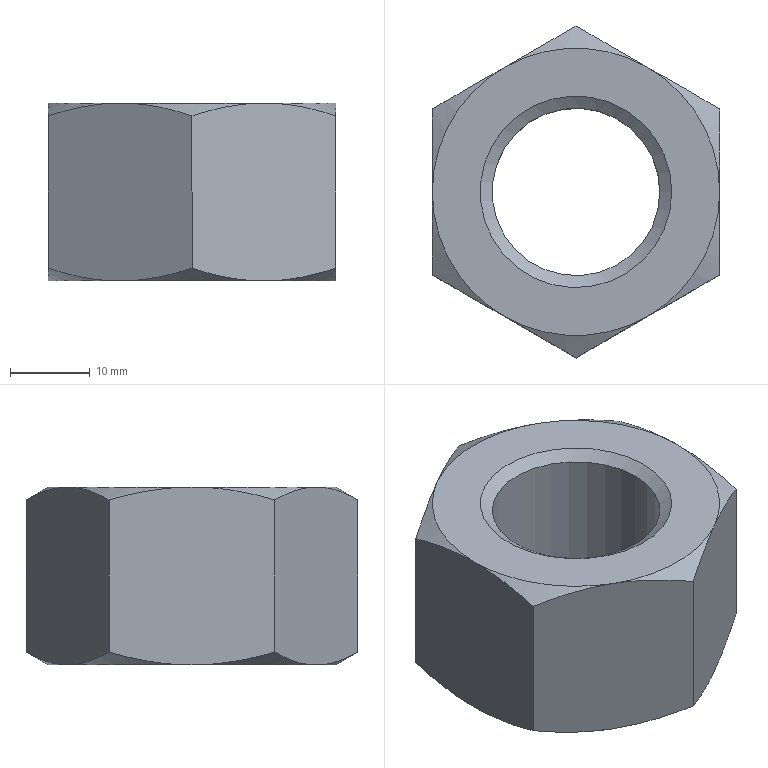Part | NX | features Hexagon Nut ISO - 4034 - M24 - N_Hexagon Nut ISO - 4034 - M24 - N 2 | 1 solid | 24 faces | box 36 x 41.569 x 22.3 mm | volume 17091 mm3 | cone 14 | plane 8 | cylinder 2 | commonest cylinder face diameters 21 x1 24 x1
STEP:
#1=CARTESIAN_POINT('',(9.,15.588,-22.3));
#2=VERTEX_POINT('',#1);
#3=CARTESIAN_POINT('',(18.,10.392,-20.692));
#4=VERTEX_POINT('',#3);
#5=CARTESIAN_POINT('',(9.,15.588,-22.3));
#6=CARTESIAN_POINT('',(12.072,13.815,-22.3));
#7=CARTESIAN_POINT('',(15.06,12.09,-21.672));
#8=CARTESIAN_POINT('',(18.,10.392,-20.692));
#9=B_SPLINE_CURVE_WITH_KNOTS('',3,(#5,#6,#7,#8),.UNSPECIFIED.,.F.,.F.,(4,4),(0.,0.01052),.UNSPECIFIED.);
#10=EDGE_CURVE('',#2,#4,#9,.T.);
#11=ORIENTED_EDGE('',*,*,#10,.F.);
#12=CARTESIAN_POINT('',(-0.000000038,20.785,-20.692));
#13=VERTEX_POINT('',#12);
#14=CARTESIAN_POINT('',(-0.000000042,20.785,-20.692));
#15=CARTESIAN_POINT('',(2.94,19.087,-21.672));
#16=CARTESIAN_POINT('',(5.928,17.362,-22.3));
#17=CARTESIAN_POINT('',(9.,15.588,-22.3));
#18=B_SPLINE_CURVE_WITH_KNOTS('',3,(#14,#15,#16,#17),.UNSPECIFIED.,.F.,.F.,(4,4),(0.,0.01052),.UNSPECIFIED.);
#19=EDGE_CURVE('',#13,#2,#18,.T.);
#20=ORIENTED_EDGE('',*,*,#19,.F.);
#21=CARTESIAN_POINT('',(0.000000012,20.785,-1.608));
#22=VERTEX_POINT('',#21);
#23=CARTESIAN_POINT('',(0.,20.785,-22.3));
#24=DIRECTION('',(0.,0.,1.));
#25=VECTOR('',#24,1000.);
#26=LINE('',#23,#25);
#27=EDGE_CURVE('',#22,#13,#26,.F.);
#28=ORIENTED_EDGE('',*,*,#27,.F.);
#29=CARTESIAN_POINT('',(9.,15.588,0.));
#30=VERTEX_POINT('',#29);
#31=CARTESIAN_POINT('',(9.,15.588,0.));
#32=CARTESIAN_POINT('',(5.928,17.362,0.));
#33=CARTESIAN_POINT('',(2.94,19.087,-0.6275));
#34=CARTESIAN_POINT('',(0.000000026,20.785,-1.608));
#35=B_SPLINE_CURVE_WITH_KNOTS('',3,(#31,#32,#33,#34),.UNSPECIFIED.,.F.,.F.,(4,4),(0.,0.01052),.UNSPECIFIED.);
#36=EDGE_CURVE('',#30,#22,#35,.T.);
#37=ORIENTED_EDGE('',*,*,#36,.F.);
#38=CARTESIAN_POINT('',(18.,10.392,-1.608));
#39=VERTEX_POINT('',#38);
#40=CARTESIAN_POINT('',(18.,10.392,-1.608));
#41=CARTESIAN_POINT('',(15.06,12.09,-0.6275));
#42=CARTESIAN_POINT('',(12.072,13.815,0.));
#43=CARTESIAN_POINT('',(9.,15.588,0.));
#44=B_SPLINE_CURVE_WITH_KNOTS('',3,(#40,#41,#42,#43),.UNSPECIFIED.,.F.,.F.,(4,4),(0.,0.01052),.UNSPECIFIED.);
#45=EDGE_CURVE('',#39,#30,#44,.T.);
#46=ORIENTED_EDGE('',*,*,#45,.F.);
#47=CARTESIAN_POINT('',(18.,10.392,-22.3));
#48=DIRECTION('',(0.,0.,1.));
#49=VECTOR('',#48,1000.);
#50=LINE('',#47,#49);
#51=EDGE_CURVE('',#39,#4,#50,.F.);
#52=ORIENTED_EDGE('',*,*,#51,.T.);
#53=EDGE_LOOP('',(#11,#20,#28,#37,#46,#52));
#54=FACE_BOUND('',#53,.T.);
#55=CARTESIAN_POINT('',(18.,10.392,-22.3));
#56=DIRECTION('',(0.5,0.866,0.));
#57=DIRECTION('',(-0.866,0.5,0.));
#58=AXIS2_PLACEMENT_3D('',#55,#56,#57);
#59=PLANE('',#58);
#60=ADVANCED_FACE('',(#54),#59,.T.);
#61=CARTESIAN_POINT('',(18.,-10.392,-20.692));
#62=VERTEX_POINT('',#61);
#63=CARTESIAN_POINT('',(18.,-10.392,-1.608));
#64=VERTEX_POINT('',#63);
#65=CARTESIAN_POINT('',(18.,-10.392,-22.3));
#66=DIRECTION('',(0.,0.,1.));
#67=VECTOR('',#66,1000.);
#68=LINE('',#65,#67);
#69=EDGE_CURVE('',#62,#64,#68,.T.);
#70=ORIENTED_EDGE('',*,*,#69,.F.);
#71=CARTESIAN_POINT('',(18.,0.,-22.3));
#72=VERTEX_POINT('',#71);
#73=CARTESIAN_POINT('',(18.,0.,-22.3));
#74=CARTESIAN_POINT('',(18.,-3.547,-22.3));
#75=CARTESIAN_POINT('',(18.,-6.997,-21.672));
#76=CARTESIAN_POINT('',(18.,-10.392,-20.692));
#77=B_SPLINE_CURVE_WITH_KNOTS('',3,(#73,#74,#75,#76),.UNSPECIFIED.,.F.,.F.,(4,4),(0.,0.01052),.UNSPECIFIED.);
#78=EDGE_CURVE('',#72,#62,#77,.T.);
#79=ORIENTED_EDGE('',*,*,#78,.F.);
#80=CARTESIAN_POINT('',(18.,10.392,-20.692));
#81=CARTESIAN_POINT('',(18.,6.997,-21.672));
#82=CARTESIAN_POINT('',(18.,3.547,-22.3));
#83=CARTESIAN_POINT('',(18.,0.,-22.3));
#84=B_SPLINE_CURVE_WITH_KNOTS('',3,(#80,#81,#82,#83),.UNSPECIFIED.,.F.,.F.,(4,4),(0.,0.01052),.UNSPECIFIED.);
#85=EDGE_CURVE('',#4,#72,#84,.T.);
#86=ORIENTED_EDGE('',*,*,#85,.F.);
#87=ORIENTED_EDGE('',*,*,#51,.F.);
#88=CARTESIAN_POINT('',(18.,0.,0.));
#89=VERTEX_POINT('',#88);
#90=CARTESIAN_POINT('',(18.,0.,0.));
#91=CARTESIAN_POINT('',(18.,3.547,0.));
#92=CARTESIAN_POINT('',(18.,6.997,-0.6275));
#93=CARTESIAN_POINT('',(18.,10.392,-1.608));
#94=B_SPLINE_CURVE_WITH_KNOTS('',3,(#90,#91,#92,#93),.UNSPECIFIED.,.F.,.F.,(4,4),(0.,0.01052),.UNSPECIFIED.);
#95=EDGE_CURVE('',#89,#39,#94,.T.);
#96=ORIENTED_EDGE('',*,*,#95,.F.);
#97=CARTESIAN_POINT('',(18.,-10.392,-1.608));
#98=CARTESIAN_POINT('',(18.,-6.997,-0.6275));
#99=CARTESIAN_POINT('',(18.,-3.547,0.));
#100=CARTESIAN_POINT('',(18.,0.,0.));
#101=B_SPLINE_CURVE_WITH_KNOTS('',3,(#97,#98,#99,#100),.UNSPECIFIED.,.F.,.F.,(4,4),(0.,0.01052),.UNSPECIFIED.);
#102=EDGE_CURVE('',#64,#89,#101,.T.);
#103=ORIENTED_EDGE('',*,*,#102,.F.);
#104=EDGE_LOOP('',(#70,#79,#86,#87,#96,#103));
#105=FACE_BOUND('',#104,.T.);
#106=CARTESIAN_POINT('',(18.,10.392,-22.3));
#107=DIRECTION('',(-1.,0.,0.));
#108=DIRECTION('',(0.,0.,1.));
#109=AXIS2_PLACEMENT_3D('',#106,#107,#108);
#110=PLANE('',#109);
#111=ADVANCED_FACE('',(#105),#110,.F.);
#112=CARTESIAN_POINT('',(9.,-15.588,-22.3));
#113=VERTEX_POINT('',#112);
#114=CARTESIAN_POINT('',(0.000000038,-20.785,-20.692));
#115=VERTEX_POINT('',#114);
#116=CARTESIAN_POINT('',(9.,-15.588,-22.3));
#117=CARTESIAN_POINT('',(5.928,-17.362,-22.3));
#118=CARTESIAN_POINT('',(2.94,-19.087,-21.672));
#119=CARTESIAN_POINT('',(0.000000075,-20.785,-20.692));
#120=B_SPLINE_CURVE_WITH_KNOTS('',3,(#116,#117,#118,#119),.UNSPECIFIED.,.F.,.F.,(4,4),(0.,0.01052),.UNSPECIFIED.);
#121=EDGE_CURVE('',#113,#115,#120,.T.);
#122=ORIENTED_EDGE('',*,*,#121,.F.);
#123=CARTESIAN_POINT('',(18.,-10.392,-20.692));
#124=CARTESIAN_POINT('',(15.06,-12.09,-21.672));
#125=CARTESIAN_POINT('',(12.072,-13.815,-22.3));
#126=CARTESIAN_POINT('',(9.,-15.588,-22.3));
#127=B_SPLINE_CURVE_WITH_KNOTS('',3,(#123,#124,#125,#126),.UNSPECIFIED.,.F.,.F.,(4,4),(0.,0.01052),.UNSPECIFIED.);
#128=EDGE_CURVE('',#62,#113,#127,.T.);
#129=ORIENTED_EDGE('',*,*,#128,.F.);
#130=ORIENTED_EDGE('',*,*,#69,.T.);
#131=CARTESIAN_POINT('',(9.,-15.588,0.));
#132=VERTEX_POINT('',#131);
#133=CARTESIAN_POINT('',(9.,-15.588,0.));
#134=CARTESIAN_POINT('',(12.072,-13.815,0.));
#135=CARTESIAN_POINT('',(15.06,-12.09,-0.6275));
#136=CARTESIAN_POINT('',(18.,-10.392,-1.608));
#137=B_SPLINE_CURVE_WITH_KNOTS('',3,(#133,#134,#135,#136),.UNSPECIFIED.,.F.,.F.,(4,4),(0.,0.01052),.UNSPECIFIED.);
#138=EDGE_CURVE('',#132,#64,#137,.T.);
#139=ORIENTED_EDGE('',*,*,#138,.F.);
#140=CARTESIAN_POINT('',(-0.000000038,-20.785,-1.608));
#141=VERTEX_POINT('',#140);
#142=CARTESIAN_POINT('',(-0.000000042,-20.785,-1.608));
#143=CARTESIAN_POINT('',(2.94,-19.087,-0.6275));
#144=CARTESIAN_POINT('',(5.928,-17.362,0.));
#145=CARTESIAN_POINT('',(9.,-15.588,0.));
#146=B_SPLINE_CURVE_WITH_KNOTS('',3,(#142,#143,#144,#145),.UNSPECIFIED.,.F.,.F.,(4,4),(0.,0.01052),.UNSPECIFIED.);
#147=EDGE_CURVE('',#141,#132,#146,.T.);
#148=ORIENTED_EDGE('',*,*,#147,.F.);
#149=CARTESIAN_POINT('',(0.,-20.785,-22.3));
#150=DIRECTION('',(0.,0.,1.));
#151=VECTOR('',#150,1000.);
#152=LINE('',#149,#151);
#153=EDGE_CURVE('',#115,#141,#152,.T.);
#154=ORIENTED_EDGE('',*,*,#153,.F.);
#155=EDGE_LOOP('',(#122,#129,#130,#139,#148,#154));
#156=FACE_BOUND('',#155,.T.);
#157=CARTESIAN_POINT('',(0.,-20.785,-22.3));
#158=DIRECTION('',(0.5,-0.866,0.));
#159=DIRECTION('',(0.866,0.5,0.));
#160=AXIS2_PLACEMENT_3D('',#157,#158,#159);
#161=PLANE('',#160);
#162=ADVANCED_FACE('',(#156),#161,.T.);
#163=CARTESIAN_POINT('',(-9.,-15.588,-22.3));
#164=VERTEX_POINT('',#163);
#165=CARTESIAN_POINT('',(-18.,-10.392,-20.692));
#166=VERTEX_POINT('',#165);
#167=CARTESIAN_POINT('',(-9.,-15.588,-22.3));
#168=CARTESIAN_POINT('',(-12.072,-13.815,-22.3));
#169=CARTESIAN_POINT('',(-15.06,-12.09,-21.672));
#170=CARTESIAN_POINT('',(-18.,-10.392,-20.692));
#171=B_SPLINE_CURVE_WITH_KNOTS('',3,(#167,#168,#169,#170),.UNSPECIFIED.,.F.,.F.,(4,4),(0.,0.01052),.UNSPECIFIED.);
#172=EDGE_CURVE('',#164,#166,#171,.T.);
#173=ORIENTED_EDGE('',*,*,#172,.F.);
#174=CARTESIAN_POINT('',(0.000000042,-20.785,-20.692));
#175=CARTESIAN_POINT('',(-2.94,-19.087,-21.672));
#176=CARTESIAN_POINT('',(-5.928,-17.362,-22.3));
#177=CARTESIAN_POINT('',(-9.,-15.588,-22.3));
#178=B_SPLINE_CURVE_WITH_KNOTS('',3,(#174,#175,#176,#177),.UNSPECIFIED.,.F.,.F.,(4,4),(0.,0.01052),.UNSPECIFIED.);
#179=EDGE_CURVE('',#115,#164,#178,.T.);
#180=ORIENTED_EDGE('',*,*,#179,.F.);
#181=ORIENTED_EDGE('',*,*,#153,.T.);
#182=CARTESIAN_POINT('',(-9.,-15.588,0.));
#183=VERTEX_POINT('',#182);
#184=CARTESIAN_POINT('',(-9.,-15.588,0.));
#185=CARTESIAN_POINT('',(-5.928,-17.362,0.));
#186=CARTESIAN_POINT('',(-2.94,-19.087,-0.6275));
#187=CARTESIAN_POINT('',(-0.000000075,-20.785,-1.608));
#188=B_SPLINE_CURVE_WITH_KNOTS('',3,(#184,#185,#186,#187),.UNSPECIFIED.,.F.,.F.,(4,4),(0.,0.01052),.UNSPECIFIED.);
#189=EDGE_CURVE('',#183,#141,#188,.T.);
#190=ORIENTED_EDGE('',*,*,#189,.F.);
#191=CARTESIAN_POINT('',(-18.,-10.392,-1.608));
#192=VERTEX_POINT('',#191);
#193=CARTESIAN_POINT('',(-18.,-10.392,-1.608));
#194=CARTESIAN_POINT('',(-15.06,-12.09,-0.6275));
#195=CARTESIAN_POINT('',(-12.072,-13.815,0.));
#196=CARTESIAN_POINT('',(-9.,-15.588,0.));
#197=B_SPLINE_CURVE_WITH_KNOTS('',3,(#193,#194,#195,#196),.UNSPECIFIED.,.F.,.F.,(4,4),(0.,0.01052),.UNSPECIFIED.);
#198=EDGE_CURVE('',#192,#183,#197,.T.);
#199=ORIENTED_EDGE('',*,*,#198,.F.);
#200=CARTESIAN_POINT('',(-18.,-10.392,-22.3));
#201=DIRECTION('',(0.,0.,1.));
#202=VECTOR('',#201,1000.);
#203=LINE('',#200,#202);
#204=EDGE_CURVE('',#166,#192,#203,.T.);
#205=ORIENTED_EDGE('',*,*,#204,.F.);
#206=EDGE_LOOP('',(#173,#180,#181,#190,#199,#205));
#207=FACE_BOUND('',#206,.T.);
#208=CARTESIAN_POINT('',(-18.,-10.392,-22.3));
#209=DIRECTION('',(-0.5,-0.866,0.));
#210=DIRECTION('',(0.866,-0.5,0.));
#211=AXIS2_PLACEMENT_3D('',#208,#209,#210);
#212=PLANE('',#211);
#213=ADVANCED_FACE('',(#207),#212,.T.);
#214=CARTESIAN_POINT('',(-18.,0.,-22.3));
#215=VERTEX_POINT('',#214);
#216=CARTESIAN_POINT('',(-18.,10.392,-20.692));
#217=VERTEX_POINT('',#216);
#218=CARTESIAN_POINT('',(-18.,0.,-22.3));
#219=CARTESIAN_POINT('',(-18.,3.547,-22.3));
#220=CARTESIAN_POINT('',(-18.,6.997,-21.672));
#221=CARTESIAN_POINT('',(-18.,10.392,-20.692));
#222=B_SPLINE_CURVE_WITH_KNOTS('',3,(#218,#219,#220,#221),.UNSPECIFIED.,.F.,.F.,(4,4),(0.,0.01052),.UNSPECIFIED.);
#223=EDGE_CURVE('',#215,#217,#222,.T.);
#224=ORIENTED_EDGE('',*,*,#223,.F.);
#225=CARTESIAN_POINT('',(-18.,-10.392,-20.692));
#226=CARTESIAN_POINT('',(-18.,-6.997,-21.672));
#227=CARTESIAN_POINT('',(-18.,-3.547,-22.3));
#228=CARTESIAN_POINT('',(-18.,0.,-22.3));
#229=B_SPLINE_CURVE_WITH_KNOTS('',3,(#225,#226,#227,#228),.UNSPECIFIED.,.F.,.F.,(4,4),(0.,0.01052),.UNSPECIFIED.);
#230=EDGE_CURVE('',#166,#215,#229,.T.);
#231=ORIENTED_EDGE('',*,*,#230,.F.);
#232=ORIENTED_EDGE('',*,*,#204,.T.);
#233=CARTESIAN_POINT('',(-18.,0.,0.));
#234=VERTEX_POINT('',#233);
#235=CARTESIAN_POINT('',(-18.,0.,0.));
#236=CARTESIAN_POINT('',(-18.,-3.547,0.));
#237=CARTESIAN_POINT('',(-18.,-6.997,-0.6275));
#238=CARTESIAN_POINT('',(-18.,-10.392,-1.608));
#239=B_SPLINE_CURVE_WITH_KNOTS('',3,(#235,#236,#237,#238),.UNSPECIFIED.,.F.,.F.,(4,4),(0.,0.01052),.UNSPECIFIED.);
#240=EDGE_CURVE('',#234,#192,#239,.T.);
#241=ORIENTED_EDGE('',*,*,#240,.F.);
#242=CARTESIAN_POINT('',(-18.,10.392,-1.608));
#243=VERTEX_POINT('',#242);
#244=CARTESIAN_POINT('',(-18.,10.392,-1.608));
#245=CARTESIAN_POINT('',(-18.,6.997,-0.6275));
#246=CARTESIAN_POINT('',(-18.,3.547,0.));
#247=CARTESIAN_POINT('',(-18.,0.,0.));
#248=B_SPLINE_CURVE_WITH_KNOTS('',3,(#244,#245,#246,#247),.UNSPECIFIED.,.F.,.F.,(4,4),(0.,0.01052),.UNSPECIFIED.);
#249=EDGE_CURVE('',#243,#234,#248,.T.);
#250=ORIENTED_EDGE('',*,*,#249,.F.);
#251=CARTESIAN_POINT('',(-18.,10.392,-22.3));
#252=DIRECTION('',(0.,0.,1.));
#253=VECTOR('',#252,1000.);
#254=LINE('',#251,#253);
#255=EDGE_CURVE('',#217,#243,#254,.T.);
#256=ORIENTED_EDGE('',*,*,#255,.F.);
#257=EDGE_LOOP('',(#224,#231,#232,#241,#250,#256));
#258=FACE_BOUND('',#257,.T.);
#259=CARTESIAN_POINT('',(-18.,10.392,-22.3));
#260=DIRECTION('',(-1.,0.,0.));
#261=DIRECTION('',(0.,0.,1.));
#262=AXIS2_PLACEMENT_3D('',#259,#260,#261);
#263=PLANE('',#262);
#264=ADVANCED_FACE('',(#258),#263,.T.);
#265=CARTESIAN_POINT('',(-9.,15.588,-22.3));
#266=VERTEX_POINT('',#265);
#267=CARTESIAN_POINT('',(-9.,15.588,-22.3));
#268=CARTESIAN_POINT('',(-5.928,17.362,-22.3));
#269=CARTESIAN_POINT('',(-2.94,19.087,-21.672));
#270=CARTESIAN_POINT('',(-0.000000075,20.785,-20.692));
#271=B_SPLINE_CURVE_WITH_KNOTS('',3,(#267,#268,#269,#270),.UNSPECIFIED.,.F.,.F.,(4,4),(0.,0.01052),.UNSPECIFIED.);
#272=EDGE_CURVE('',#266,#13,#271,.T.);
#273=ORIENTED_EDGE('',*,*,#272,.F.);
#274=CARTESIAN_POINT('',(-18.,10.392,-20.692));
#275=CARTESIAN_POINT('',(-15.06,12.09,-21.672));
#276=CARTESIAN_POINT('',(-12.072,13.815,-22.3));
#277=CARTESIAN_POINT('',(-9.,15.588,-22.3));
#278=B_SPLINE_CURVE_WITH_KNOTS('',3,(#274,#275,#276,#277),.UNSPECIFIED.,.F.,.F.,(4,4),(0.,0.01052),.UNSPECIFIED.);
#279=EDGE_CURVE('',#217,#266,#278,.T.);
#280=ORIENTED_EDGE('',*,*,#279,.F.);
#281=ORIENTED_EDGE('',*,*,#255,.T.);
#282=CARTESIAN_POINT('',(-9.,15.588,0.));
#283=VERTEX_POINT('',#282);
#284=CARTESIAN_POINT('',(-9.,15.588,0.));
#285=CARTESIAN_POINT('',(-12.072,13.815,0.));
#286=CARTESIAN_POINT('',(-15.06,12.09,-0.6275));
#287=CARTESIAN_POINT('',(-18.,10.392,-1.608));
#288=B_SPLINE_CURVE_WITH_KNOTS('',3,(#284,#285,#286,#287),.UNSPECIFIED.,.F.,.F.,(4,4),(0.,0.01052),.UNSPECIFIED.);
#289=EDGE_CURVE('',#283,#243,#288,.T.);
#290=ORIENTED_EDGE('',*,*,#289,.F.);
#291=CARTESIAN_POINT('',(-0.000000017,20.785,-1.608));
#292=CARTESIAN_POINT('',(-2.94,19.087,-0.6275));
#293=CARTESIAN_POINT('',(-5.928,17.362,0.));
#294=CARTESIAN_POINT('',(-9.,15.588,0.));
#295=B_SPLINE_CURVE_WITH_KNOTS('',3,(#291,#292,#293,#294),.UNSPECIFIED.,.F.,.F.,(4,4),(0.,0.01052),.UNSPECIFIED.);
#296=EDGE_CURVE('',#22,#283,#295,.T.);
#297=ORIENTED_EDGE('',*,*,#296,.F.);
#298=ORIENTED_EDGE('',*,*,#27,.T.);
#299=EDGE_LOOP('',(#273,#280,#281,#290,#297,#298));
#300=FACE_BOUND('',#299,.T.);
#301=CARTESIAN_POINT('',(0.,20.785,-22.3));
#302=DIRECTION('',(-0.5,0.866,0.));
#303=DIRECTION('',(-0.866,-0.5,0.));
#304=AXIS2_PLACEMENT_3D('',#301,#302,#303);
#305=PLANE('',#304);
#306=ADVANCED_FACE('',(#300),#305,.T.);
#307=ORIENTED_EDGE('',*,*,#230,.T.);
#308=CARTESIAN_POINT('',(0.,0.,-22.3));
#309=DIRECTION('',(0.,0.,1.));
#310=DIRECTION('',(0.,-1.,0.));
#311=AXIS2_PLACEMENT_3D('',#308,#309,#310);
#312=CIRCLE('',#311,18.);
#313=EDGE_CURVE('',#164,#215,#312,.F.);
#314=ORIENTED_EDGE('',*,*,#313,.F.);
#315=ORIENTED_EDGE('',*,*,#172,.T.);
#316=EDGE_LOOP('',(#307,#314,#315));
#317=FACE_BOUND('',#316,.T.);
#318=CARTESIAN_POINT('',(0.,0.,-20.683));
#319=DIRECTION('',(0.,0.,1.));
#320=DIRECTION('',(0.,-1.,0.));
#321=AXIS2_PLACEMENT_3D('',#318,#319,#320);
#322=CONICAL_SURFACE('',#321,20.801,1.047);
#323=ADVANCED_FACE('',(#317),#322,.T.);
#324=CARTESIAN_POINT('',(0.,0.,-22.3));
#325=DIRECTION('',(0.,0.,1.));
#326=DIRECTION('',(0.,-1.,0.));
#327=AXIS2_PLACEMENT_3D('',#324,#325,#326);
#328=CIRCLE('',#327,18.);
#329=EDGE_CURVE('',#215,#266,#328,.F.);
#330=ORIENTED_EDGE('',*,*,#329,.F.);
#331=ORIENTED_EDGE('',*,*,#223,.T.);
#332=ORIENTED_EDGE('',*,*,#279,.T.);
#333=EDGE_LOOP('',(#330,#331,#332));
#334=FACE_BOUND('',#333,.T.);
#335=CARTESIAN_POINT('',(0.,0.,-20.683));
#336=DIRECTION('',(0.,0.,1.));
#337=DIRECTION('',(0.,-1.,0.));
#338=AXIS2_PLACEMENT_3D('',#335,#336,#337);
#339=CONICAL_SURFACE('',#338,20.801,1.047);
#340=ADVANCED_FACE('',(#334),#339,.T.);
#341=ORIENTED_EDGE('',*,*,#19,.T.);
#342=CARTESIAN_POINT('',(0.,0.,-22.3));
#343=DIRECTION('',(0.,0.,1.));
#344=DIRECTION('',(1.,0.,0.));
#345=AXIS2_PLACEMENT_3D('',#342,#343,#344);
#346=CIRCLE('',#345,18.);
#347=EDGE_CURVE('',#266,#2,#346,.F.);
#348=ORIENTED_EDGE('',*,*,#347,.F.);
#349=ORIENTED_EDGE('',*,*,#272,.T.);
#350=EDGE_LOOP('',(#341,#348,#349));
#351=FACE_BOUND('',#350,.T.);
#352=CARTESIAN_POINT('',(0.,0.,-20.683));
#353=DIRECTION('',(0.,0.,1.));
#354=DIRECTION('',(1.,0.,0.));
#355=AXIS2_PLACEMENT_3D('',#352,#353,#354);
#356=CONICAL_SURFACE('',#355,20.801,1.047);
#357=ADVANCED_FACE('',(#351),#356,.T.);
#358=ORIENTED_EDGE('',*,*,#85,.T.);
#359=CARTESIAN_POINT('',(0.,0.,-22.3));
#360=DIRECTION('',(0.,0.,1.));
#361=DIRECTION('',(0.,-1.,0.));
#362=AXIS2_PLACEMENT_3D('',#359,#360,#361);
#363=CIRCLE('',#362,18.);
#364=EDGE_CURVE('',#2,#72,#363,.F.);
#365=ORIENTED_EDGE('',*,*,#364,.F.);
#366=ORIENTED_EDGE('',*,*,#10,.T.);
#367=EDGE_LOOP('',(#358,#365,#366));
#368=FACE_BOUND('',#367,.T.);
#369=CARTESIAN_POINT('',(0.,0.,-20.683));
#370=DIRECTION('',(0.,0.,1.));
#371=DIRECTION('',(0.,-1.,0.));
#372=AXIS2_PLACEMENT_3D('',#369,#370,#371);
#373=CONICAL_SURFACE('',#372,20.801,1.047);
#374=ADVANCED_FACE('',(#368),#373,.T.);
#375=CARTESIAN_POINT('',(0.,0.,-22.3));
#376=DIRECTION('',(0.,0.,1.));
#377=DIRECTION('',(1.,0.,0.));
#378=AXIS2_PLACEMENT_3D('',#375,#376,#377);
#379=CIRCLE('',#378,18.);
#380=EDGE_CURVE('',#72,#113,#379,.F.);
#381=ORIENTED_EDGE('',*,*,#380,.F.);
#382=ORIENTED_EDGE('',*,*,#78,.T.);
#383=ORIENTED_EDGE('',*,*,#128,.T.);
#384=EDGE_LOOP('',(#381,#382,#383));
#385=FACE_BOUND('',#384,.T.);
#386=CARTESIAN_POINT('',(0.,0.,-20.683));
#387=DIRECTION('',(0.,0.,1.));
#388=DIRECTION('',(1.,0.,0.));
#389=AXIS2_PLACEMENT_3D('',#386,#387,#388);
#390=CONICAL_SURFACE('',#389,20.801,1.047);
#391=ADVANCED_FACE('',(#385),#390,.T.);
#392=ORIENTED_EDGE('',*,*,#179,.T.);
#393=CARTESIAN_POINT('',(0.,0.,-22.3));
#394=DIRECTION('',(0.,0.,1.));
#395=DIRECTION('',(1.,0.,0.));
#396=AXIS2_PLACEMENT_3D('',#393,#394,#395);
#397=CIRCLE('',#396,18.);
#398=EDGE_CURVE('',#113,#164,#397,.F.);
#399=ORIENTED_EDGE('',*,*,#398,.F.);
#400=ORIENTED_EDGE('',*,*,#121,.T.);
#401=EDGE_LOOP('',(#392,#399,#400));
#402=FACE_BOUND('',#401,.T.);
#403=CARTESIAN_POINT('',(0.,0.,-20.683));
#404=DIRECTION('',(0.,0.,1.));
#405=DIRECTION('',(1.,0.,0.));
#406=AXIS2_PLACEMENT_3D('',#403,#404,#405);
#407=CONICAL_SURFACE('',#406,20.801,1.047);
#408=ADVANCED_FACE('',(#402),#407,.T.);
#409=ORIENTED_EDGE('',*,*,#36,.T.);
#410=ORIENTED_EDGE('',*,*,#296,.T.);
#411=CARTESIAN_POINT('',(0.,0.,0.));
#412=DIRECTION('',(0.,0.,-1.));
#413=DIRECTION('',(0.,1.,0.));
#414=AXIS2_PLACEMENT_3D('',#411,#412,#413);
#415=CIRCLE('',#414,18.);
#416=EDGE_CURVE('',#283,#30,#415,.T.);
#417=ORIENTED_EDGE('',*,*,#416,.T.);
#418=EDGE_LOOP('',(#409,#410,#417));
#419=FACE_BOUND('',#418,.T.);
#420=CARTESIAN_POINT('',(0.,0.,-1.617));
#421=DIRECTION('',(0.,0.,-1.));
#422=DIRECTION('',(0.,1.,0.));
#423=AXIS2_PLACEMENT_3D('',#420,#421,#422);
#424=CONICAL_SURFACE('',#423,20.801,1.047);
#425=ADVANCED_FACE('',(#419),#424,.T.);
#426=ORIENTED_EDGE('',*,*,#95,.T.);
#427=ORIENTED_EDGE('',*,*,#45,.T.);
#428=CARTESIAN_POINT('',(0.,0.,0.));
#429=DIRECTION('',(0.,0.,-1.));
#430=DIRECTION('',(0.,1.,0.));
#431=AXIS2_PLACEMENT_3D('',#428,#429,#430);
#432=CIRCLE('',#431,18.);
#433=EDGE_CURVE('',#30,#89,#432,.T.);
#434=ORIENTED_EDGE('',*,*,#433,.T.);
#435=EDGE_LOOP('',(#426,#427,#434));
#436=FACE_BOUND('',#435,.T.);
#437=CARTESIAN_POINT('',(0.,0.,-1.617));
#438=DIRECTION('',(0.,0.,-1.));
#439=DIRECTION('',(0.,1.,0.));
#440=AXIS2_PLACEMENT_3D('',#437,#438,#439);
#441=CONICAL_SURFACE('',#440,20.801,1.047);
#442=ADVANCED_FACE('',(#436),#441,.T.);
#443=CARTESIAN_POINT('',(0.,0.,0.));
#444=DIRECTION('',(0.,0.,-1.));
#445=DIRECTION('',(0.,1.,0.));
#446=AXIS2_PLACEMENT_3D('',#443,#444,#445);
#447=CIRCLE('',#446,18.);
#448=EDGE_CURVE('',#89,#132,#447,.T.);
#449=ORIENTED_EDGE('',*,*,#448,.T.);
#450=ORIENTED_EDGE('',*,*,#138,.T.);
#451=ORIENTED_EDGE('',*,*,#102,.T.);
#452=EDGE_LOOP('',(#449,#450,#451));
#453=FACE_BOUND('',#452,.T.);
#454=CARTESIAN_POINT('',(0.,0.,-1.617));
#455=DIRECTION('',(0.,0.,-1.));
#456=DIRECTION('',(0.,1.,0.));
#457=AXIS2_PLACEMENT_3D('',#454,#455,#456);
#458=CONICAL_SURFACE('',#457,20.801,1.047);
#459=ADVANCED_FACE('',(#453),#458,.T.);
#460=ORIENTED_EDGE('',*,*,#189,.T.);
#461=ORIENTED_EDGE('',*,*,#147,.T.);
#462=CARTESIAN_POINT('',(0.,0.,0.));
#463=DIRECTION('',(0.,0.,-1.));
#464=DIRECTION('',(0.,1.,0.));
#465=AXIS2_PLACEMENT_3D('',#462,#463,#464);
#466=CIRCLE('',#465,18.);
#467=EDGE_CURVE('',#132,#183,#466,.T.);
#468=ORIENTED_EDGE('',*,*,#467,.T.);
#469=EDGE_LOOP('',(#460,#461,#468));
#470=FACE_BOUND('',#469,.T.);
#471=CARTESIAN_POINT('',(0.,0.,-1.617));
#472=DIRECTION('',(0.,0.,-1.));
#473=DIRECTION('',(0.,1.,0.));
#474=AXIS2_PLACEMENT_3D('',#471,#472,#473);
#475=CONICAL_SURFACE('',#474,20.801,1.047);
#476=ADVANCED_FACE('',(#470),#475,.T.);
#477=ORIENTED_EDGE('',*,*,#240,.T.);
#478=ORIENTED_EDGE('',*,*,#198,.T.);
#479=CARTESIAN_POINT('',(0.,0.,0.));
#480=DIRECTION('',(0.,0.,-1.));
#481=DIRECTION('',(0.,1.,0.));
#482=AXIS2_PLACEMENT_3D('',#479,#480,#481);
#483=CIRCLE('',#482,18.);
#484=EDGE_CURVE('',#183,#234,#483,.T.);
#485=ORIENTED_EDGE('',*,*,#484,.T.);
#486=EDGE_LOOP('',(#477,#478,#485));
#487=FACE_BOUND('',#486,.T.);
#488=CARTESIAN_POINT('',(0.,0.,-1.617));
#489=DIRECTION('',(0.,0.,-1.));
#490=DIRECTION('',(0.,1.,0.));
#491=AXIS2_PLACEMENT_3D('',#488,#489,#490);
#492=CONICAL_SURFACE('',#491,20.801,1.047);
#493=ADVANCED_FACE('',(#487),#492,.T.);
#494=CARTESIAN_POINT('',(0.,0.,0.));
#495=DIRECTION('',(0.,0.,-1.));
#496=DIRECTION('',(0.,1.,0.));
#497=AXIS2_PLACEMENT_3D('',#494,#495,#496);
#498=CIRCLE('',#497,18.);
#499=EDGE_CURVE('',#234,#283,#498,.T.);
#500=ORIENTED_EDGE('',*,*,#499,.T.);
#501=ORIENTED_EDGE('',*,*,#289,.T.);
#502=ORIENTED_EDGE('',*,*,#249,.T.);
#503=EDGE_LOOP('',(#500,#501,#502));
#504=FACE_BOUND('',#503,.T.);
#505=CARTESIAN_POINT('',(0.,0.,-1.617));
#506=DIRECTION('',(0.,0.,-1.));
#507=DIRECTION('',(0.,1.,0.));
#508=AXIS2_PLACEMENT_3D('',#505,#506,#507);
#509=CONICAL_SURFACE('',#508,20.801,1.047);
#510=ADVANCED_FACE('',(#504),#509,.T.);
#511=CARTESIAN_POINT('',(12.,0.,-22.3));
#512=VERTEX_POINT('',#511);
#513=CARTESIAN_POINT('',(0.,0.,-22.3));
#514=DIRECTION('',(0.,0.,1.));
#515=DIRECTION('',(1.,0.,0.));
#516=AXIS2_PLACEMENT_3D('',#513,#514,#515);
#517=CIRCLE('',#516,12.);
#518=EDGE_CURVE('',#512,#512,#517,.T.);
#519=ORIENTED_EDGE('',*,*,#518,.T.);
#520=EDGE_LOOP('',(#519));
#521=FACE_BOUND('',#520,.T.);
#522=ORIENTED_EDGE('',*,*,#380,.T.);
#523=ORIENTED_EDGE('',*,*,#398,.T.);
#524=ORIENTED_EDGE('',*,*,#313,.T.);
#525=ORIENTED_EDGE('',*,*,#329,.T.);
#526=ORIENTED_EDGE('',*,*,#347,.T.);
#527=ORIENTED_EDGE('',*,*,#364,.T.);
#528=EDGE_LOOP('',(#522,#523,#524,#525,#526,#527));
#529=FACE_BOUND('',#528,.T.);
#530=CARTESIAN_POINT('',(0.,20.785,-22.3));
#531=DIRECTION('',(0.,0.,-1.));
#532=DIRECTION('',(-1.,0.,0.));
#533=AXIS2_PLACEMENT_3D('',#530,#531,#532);
#534=PLANE('',#533);
#535=ADVANCED_FACE('',(#521,#529),#534,.T.);
#536=CARTESIAN_POINT('',(12.,0.,0.));
#537=VERTEX_POINT('',#536);
#538=CARTESIAN_POINT('',(0.,0.,0.));
#539=DIRECTION('',(0.,0.,1.));
#540=DIRECTION('',(1.,0.,0.));
#541=AXIS2_PLACEMENT_3D('',#538,#539,#540);
#542=CIRCLE('',#541,12.);
#543=EDGE_CURVE('',#537,#537,#542,.F.);
#544=ORIENTED_EDGE('',*,*,#543,.T.);
#545=EDGE_LOOP('',(#544));
#546=FACE_BOUND('',#545,.T.);
#547=ORIENTED_EDGE('',*,*,#484,.F.);
#548=ORIENTED_EDGE('',*,*,#467,.F.);
#549=ORIENTED_EDGE('',*,*,#448,.F.);
#550=ORIENTED_EDGE('',*,*,#433,.F.);
#551=ORIENTED_EDGE('',*,*,#416,.F.);
#552=ORIENTED_EDGE('',*,*,#499,.F.);
#553=EDGE_LOOP('',(#547,#548,#549,#550,#551,#552));
#554=FACE_BOUND('',#553,.T.);
#555=CARTESIAN_POINT('',(0.,20.785,0.));
#556=DIRECTION('',(0.,0.,-1.));
#557=DIRECTION('',(-1.,0.,0.));
#558=AXIS2_PLACEMENT_3D('',#555,#556,#557);
#559=PLANE('',#558);
#560=ADVANCED_FACE('',(#546,#554),#559,.F.);
#561=CARTESIAN_POINT('',(-12.,0.,-22.275));
#562=VERTEX_POINT('',#561);
#563=CARTESIAN_POINT('',(0.,0.,-22.275));
#564=DIRECTION('',(0.,0.,-1.));
#565=DIRECTION('',(-1.,0.,0.));
#566=AXIS2_PLACEMENT_3D('',#563,#564,#565);
#567=CIRCLE('',#566,12.);
#568=EDGE_CURVE('',#562,#562,#567,.F.);
#569=ORIENTED_EDGE('',*,*,#568,.T.);
#570=EDGE_LOOP('',(#569));
#571=FACE_BOUND('',#570,.T.);
#572=ORIENTED_EDGE('',*,*,#518,.F.);
#573=EDGE_LOOP('',(#572));
#574=FACE_BOUND('',#573,.T.);
#575=CARTESIAN_POINT('',(0.,0.,-25.038));
#576=DIRECTION('',(0.,0.,1.));
#577=DIRECTION('',(1.,0.,0.));
#578=AXIS2_PLACEMENT_3D('',#575,#576,#577);
#579=CYLINDRICAL_SURFACE('',#578,12.);
#580=ADVANCED_FACE('',(#571,#574),#579,.F.);
#581=ORIENTED_EDGE('',*,*,#543,.F.);
#582=EDGE_LOOP('',(#581));
#583=FACE_BOUND('',#582,.T.);
#584=CARTESIAN_POINT('',(10.5,0.,-1.05));
#585=VERTEX_POINT('',#584);
#586=CARTESIAN_POINT('',(0.,0.,-1.05));
#587=DIRECTION('',(0.,0.,1.));
#588=DIRECTION('',(1.,0.,0.));
#589=AXIS2_PLACEMENT_3D('',#586,#587,#588);
#590=CIRCLE('',#589,10.5);
#591=EDGE_CURVE('',#585,#585,#590,.F.);
#592=ORIENTED_EDGE('',*,*,#591,.T.);
#593=EDGE_LOOP('',(#592));
#594=FACE_BOUND('',#593,.T.);
#595=CARTESIAN_POINT('',(0.,0.,0.));
#596=DIRECTION('',(0.,0.,1.));
#597=DIRECTION('',(1.,0.,0.));
#598=AXIS2_PLACEMENT_3D('',#595,#596,#597);
#599=CONICAL_SURFACE('',#598,12.,0.9599);
#600=ADVANCED_FACE('',(#583,#594),#599,.F.);
#601=ORIENTED_EDGE('',*,*,#568,.F.);
#602=EDGE_LOOP('',(#601));
#603=FACE_BOUND('',#602,.T.);
#604=CARTESIAN_POINT('',(10.5,0.,-21.224));
#605=VERTEX_POINT('',#604);
#606=CARTESIAN_POINT('',(0.,0.,-21.224));
#607=DIRECTION('',(0.,0.,1.));
#608=DIRECTION('',(1.,0.,0.));
#609=AXIS2_PLACEMENT_3D('',#606,#607,#608);
#610=CIRCLE('',#609,10.5);
#611=EDGE_CURVE('',#605,#605,#610,.T.);
#612=ORIENTED_EDGE('',*,*,#611,.T.);
#613=EDGE_LOOP('',(#612));
#614=FACE_BOUND('',#613,.T.);
#615=CARTESIAN_POINT('',(0.,0.,-22.275));
#616=DIRECTION('',(0.,0.,-1.));
#617=DIRECTION('',(-1.,0.,0.));
#618=AXIS2_PLACEMENT_3D('',#615,#616,#617);
#619=CONICAL_SURFACE('',#618,12.,0.9599);
#620=ADVANCED_FACE('',(#603,#614),#619,.F.);
#621=ORIENTED_EDGE('',*,*,#591,.F.);
#622=EDGE_LOOP('',(#621));
#623=FACE_BOUND('',#622,.T.);
#624=ORIENTED_EDGE('',*,*,#611,.F.);
#625=EDGE_LOOP('',(#624));
#626=FACE_BOUND('',#625,.T.);
#627=CARTESIAN_POINT('',(0.,0.,-22.3));
#628=DIRECTION('',(0.,0.,1.));
#629=DIRECTION('',(1.,0.,0.));
#630=AXIS2_PLACEMENT_3D('',#627,#628,#629);
#631=CYLINDRICAL_SURFACE('',#630,10.5);
#632=ADVANCED_FACE('',(#623,#626),#631,.F.);
#633=CLOSED_SHELL('',(#60,#111,#162,#213,#264,#306,#323,#340,#357,#374,#391,#408,#425,#442,#459,#476,#493,#510,#535,#560,#580,#600,#620,#632));
#634=MANIFOLD_SOLID_BREP('',#633);
#635=(LENGTH_UNIT()NAMED_UNIT(*)SI_UNIT(.MILLI.,.METRE.));
#636=UNCERTAINTY_MEASURE_WITH_UNIT(LENGTH_MEASURE(0.0508),#635,'','');
#637=(NAMED_UNIT(*)PLANE_ANGLE_UNIT()SI_UNIT($,.RADIAN.));
#638=(NAMED_UNIT(*)SI_UNIT($,.STERADIAN.)SOLID_ANGLE_UNIT());
#639=(GEOMETRIC_REPRESENTATION_CONTEXT(3)GLOBAL_UNCERTAINTY_ASSIGNED_CONTEXT((#636))GLOBAL_UNIT_ASSIGNED_CONTEXT((#635,#637,#638))REPRESENTATION_CONTEXT('',''));
#640=ADVANCED_BREP_SHAPE_REPRESENTATION('',(#634),#639);